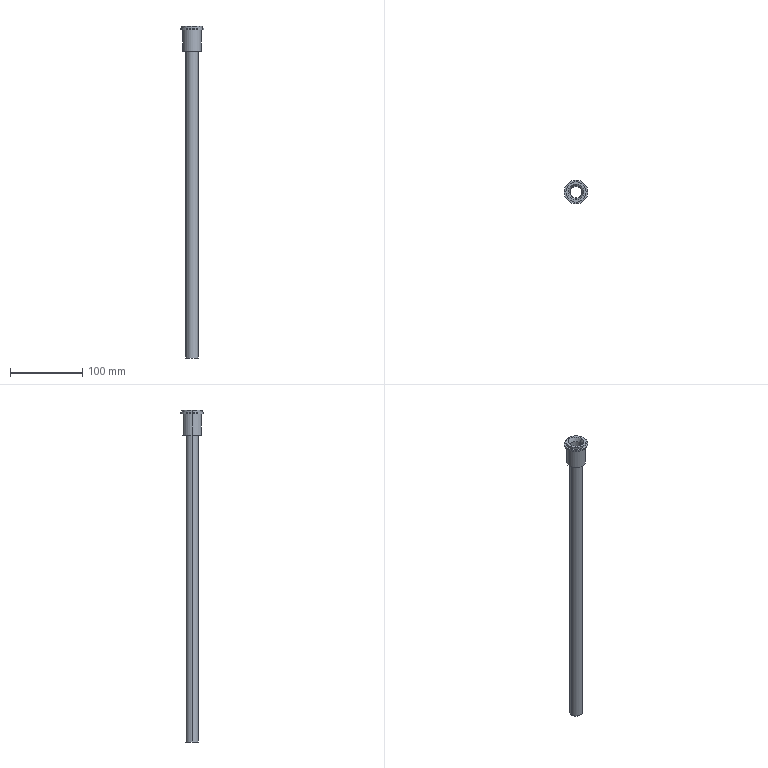Part | STEP file | Discharge pipe joint | 2 solids | 20 faces | box 33 x 33 x 460 mm | volume 22117 mm3 | cylinder 12 | plane 6 | cone 2 | commonest cylinder face diameters 17 x4 16 x2 26 x2 28 x2 33 x2
STEP:
#1=CARTESIAN_POINT('',(0.,0.,0.));
#2=DIRECTION('',(0.,0.,1.));
#3=DIRECTION('',(1.,0.,0.));
#4=AXIS2_PLACEMENT_3D('',#1,#2,#3);
#5=CARTESIAN_POINT('',(8.5,0.,-1.));
#6=VERTEX_POINT('',#5);
#7=CARTESIAN_POINT('',(11.,0.,5.));
#8=VERTEX_POINT('',#7);
#9=CARTESIAN_POINT('',(8.5,0.,-1.));
#10=DIRECTION('',(0.3846,0.,0.9231));
#11=VECTOR('',#10,1.);
#12=LINE('',#9,#11);
#13=CARTESIAN_POINT('',(0.,0.,-1.));
#14=DIRECTION('',(0.,0.,1.));
#15=DIRECTION('',(1.,0.,0.));
#16=AXIS2_PLACEMENT_3D('',#13,#14,#15);
#17=CONICAL_SURFACE('',#16,8.5,0.3948);
#18=CARTESIAN_POINT('',(6.283,0.));
#19=DIRECTION('',(0.,1.));
#20=VECTOR('',#19,1.);
#21=LINE('',#18,#20);
#22=(GEOMETRIC_REPRESENTATION_CONTEXT(2)PARAMETRIC_REPRESENTATION_CONTEXT()REPRESENTATION_CONTEXT('',''));
#23=DEFINITIONAL_REPRESENTATION('',(#21),#22);
#24=PCURVE('',#17,#23);
#25=CARTESIAN_POINT('',(0.,0.,-1.));
#26=DIRECTION('',(0.,0.,1.));
#27=DIRECTION('',(1.,0.,0.));
#28=AXIS2_PLACEMENT_3D('',#25,#26,#27);
#29=CONICAL_SURFACE('',#28,8.5,0.3948);
#30=CARTESIAN_POINT('',(0.,0.));
#31=DIRECTION('',(0.,1.));
#32=VECTOR('',#31,1.);
#33=LINE('',#30,#32);
#34=(GEOMETRIC_REPRESENTATION_CONTEXT(2)PARAMETRIC_REPRESENTATION_CONTEXT()REPRESENTATION_CONTEXT('',''));
#35=DEFINITIONAL_REPRESENTATION('',(#33),#34);
#36=PCURVE('',#29,#35);
#37=SURFACE_CURVE('',#12,(#24,#36),.PCURVE_S1.);
#38=EDGE_CURVE('',#6,#8,#37,.T.);
#39=ORIENTED_EDGE('',*,*,#38,.T.);
#40=CARTESIAN_POINT('',(-11.,0.,5.));
#41=VERTEX_POINT('',#40);
#42=CARTESIAN_POINT('',(0.,0.,5.));
#43=DIRECTION('',(0.,0.,1.));
#44=DIRECTION('',(1.,0.,0.));
#45=AXIS2_PLACEMENT_3D('',#42,#43,#44);
#46=CIRCLE('',#45,11.);
#47=CARTESIAN_POINT('',(0.,6.));
#48=DIRECTION('',(1.,0.));
#49=VECTOR('',#48,1.);
#50=LINE('',#47,#49);
#51=(GEOMETRIC_REPRESENTATION_CONTEXT(2)PARAMETRIC_REPRESENTATION_CONTEXT()REPRESENTATION_CONTEXT('',''));
#52=DEFINITIONAL_REPRESENTATION('',(#50),#51);
#53=PCURVE('',#17,#52);
#54=CARTESIAN_POINT('',(0.,0.,5.));
#55=DIRECTION('',(0.,0.,1.));
#56=DIRECTION('',(1.,0.,0.));
#57=AXIS2_PLACEMENT_3D('',#54,#55,#56);
#58=PLANE('',#57);
#59=CARTESIAN_POINT('',(0.,0.));
#60=DIRECTION('',(1.,0.));
#61=AXIS2_PLACEMENT_2D('',#59,#60);
#62=CIRCLE('',#61,11.);
#63=(GEOMETRIC_REPRESENTATION_CONTEXT(2)PARAMETRIC_REPRESENTATION_CONTEXT()REPRESENTATION_CONTEXT('',''));
#64=DEFINITIONAL_REPRESENTATION('',(#62),#63);
#65=PCURVE('',#58,#64);
#66=SURFACE_CURVE('',#46,(#53,#65),.PCURVE_S1.);
#67=EDGE_CURVE('',#41,#8,#66,.T.);
#68=ORIENTED_EDGE('',*,*,#67,.F.);
#69=CARTESIAN_POINT('',(-8.5,0.,-1.));
#70=VERTEX_POINT('',#69);
#71=CARTESIAN_POINT('',(-8.5,0.,-1.));
#72=DIRECTION('',(-0.3846,0.,0.9231));
#73=VECTOR('',#72,1.);
#74=LINE('',#71,#73);
#75=CARTESIAN_POINT('',(3.142,0.));
#76=DIRECTION('',(0.,1.));
#77=VECTOR('',#76,1.);
#78=LINE('',#75,#77);
#79=(GEOMETRIC_REPRESENTATION_CONTEXT(2)PARAMETRIC_REPRESENTATION_CONTEXT()REPRESENTATION_CONTEXT('',''));
#80=DEFINITIONAL_REPRESENTATION('',(#78),#79);
#81=PCURVE('',#17,#80);
#82=CARTESIAN_POINT('',(3.142,0.));
#83=DIRECTION('',(0.,1.));
#84=VECTOR('',#83,1.);
#85=LINE('',#82,#84);
#86=(GEOMETRIC_REPRESENTATION_CONTEXT(2)PARAMETRIC_REPRESENTATION_CONTEXT()REPRESENTATION_CONTEXT('',''));
#87=DEFINITIONAL_REPRESENTATION('',(#85),#86);
#88=PCURVE('',#29,#87);
#89=SURFACE_CURVE('',#74,(#81,#88),.PCURVE_S1.);
#90=EDGE_CURVE('',#70,#41,#89,.T.);
#91=ORIENTED_EDGE('',*,*,#90,.F.);
#92=CARTESIAN_POINT('',(0.,0.,-1.));
#93=DIRECTION('',(0.,0.,1.));
#94=DIRECTION('',(1.,0.,0.));
#95=AXIS2_PLACEMENT_3D('',#92,#93,#94);
#96=CIRCLE('',#95,8.5);
#97=CARTESIAN_POINT('',(0.,0.));
#98=DIRECTION('',(1.,0.));
#99=VECTOR('',#98,1.);
#100=LINE('',#97,#99);
#101=(GEOMETRIC_REPRESENTATION_CONTEXT(2)PARAMETRIC_REPRESENTATION_CONTEXT()REPRESENTATION_CONTEXT('',''));
#102=DEFINITIONAL_REPRESENTATION('',(#100),#101);
#103=PCURVE('',#17,#102);
#104=CARTESIAN_POINT('',(0.,0.,5.));
#105=DIRECTION('',(0.,0.,-1.));
#106=DIRECTION('',(-1.,0.,0.));
#107=AXIS2_PLACEMENT_3D('',#104,#105,#106);
#108=CYLINDRICAL_SURFACE('',#107,8.5);
#109=CARTESIAN_POINT('',(9.425,6.));
#110=DIRECTION('',(-1.,0.));
#111=VECTOR('',#110,1.);
#112=LINE('',#109,#111);
#113=(GEOMETRIC_REPRESENTATION_CONTEXT(2)PARAMETRIC_REPRESENTATION_CONTEXT()REPRESENTATION_CONTEXT('',''));
#114=DEFINITIONAL_REPRESENTATION('',(#112),#113);
#115=PCURVE('',#108,#114);
#116=SURFACE_CURVE('',#96,(#103,#115),.PCURVE_S1.);
#117=EDGE_CURVE('',#70,#6,#116,.T.);
#118=ORIENTED_EDGE('',*,*,#117,.T.);
#119=EDGE_LOOP('',(#39,#68,#91,#118));
#120=FACE_BOUND('',#119,.F.);
#121=ADVANCED_FACE('',(#120),#17,.F.);
#122=CARTESIAN_POINT('',(-13.,0.,-30.));
#123=VERTEX_POINT('',#122);
#124=CARTESIAN_POINT('',(13.,0.,-30.));
#125=VERTEX_POINT('',#124);
#126=CARTESIAN_POINT('',(0.,0.,-30.));
#127=DIRECTION('',(0.,0.,-1.));
#128=DIRECTION('',(-1.,0.,0.));
#129=AXIS2_PLACEMENT_3D('',#126,#127,#128);
#130=CIRCLE('',#129,13.);
#131=CARTESIAN_POINT('',(0.,0.,-30.));
#132=DIRECTION('',(0.,0.,1.));
#133=DIRECTION('',(1.,0.,0.));
#134=AXIS2_PLACEMENT_3D('',#131,#132,#133);
#135=CYLINDRICAL_SURFACE('',#134,13.);
#136=CARTESIAN_POINT('',(3.142,0.));
#137=DIRECTION('',(-1.,0.));
#138=VECTOR('',#137,1.);
#139=LINE('',#136,#138);
#140=(GEOMETRIC_REPRESENTATION_CONTEXT(2)PARAMETRIC_REPRESENTATION_CONTEXT()REPRESENTATION_CONTEXT('',''));
#141=DEFINITIONAL_REPRESENTATION('',(#139),#140);
#142=PCURVE('',#135,#141);
#143=CARTESIAN_POINT('',(0.,0.,-30.));
#144=DIRECTION('',(0.,0.,-1.));
#145=DIRECTION('',(-1.,0.,0.));
#146=AXIS2_PLACEMENT_3D('',#143,#144,#145);
#147=PLANE('',#146);
#148=CARTESIAN_POINT('',(0.,0.));
#149=DIRECTION('',(1.,0.));
#150=AXIS2_PLACEMENT_2D('',#148,#149);
#151=CIRCLE('',#150,13.);
#152=(GEOMETRIC_REPRESENTATION_CONTEXT(2)PARAMETRIC_REPRESENTATION_CONTEXT()REPRESENTATION_CONTEXT('',''));
#153=DEFINITIONAL_REPRESENTATION('',(#151),#152);
#154=PCURVE('',#147,#153);
#155=SURFACE_CURVE('',#130,(#142,#154),.PCURVE_S1.);
#156=EDGE_CURVE('',#123,#125,#155,.T.);
#157=ORIENTED_EDGE('',*,*,#156,.F.);
#158=CARTESIAN_POINT('',(-13.,0.,0.));
#159=VERTEX_POINT('',#158);
#160=CARTESIAN_POINT('',(-13.,0.,-30.));
#161=DIRECTION('',(0.,0.,1.));
#162=VECTOR('',#161,1.);
#163=LINE('',#160,#162);
#164=CARTESIAN_POINT('',(3.142,0.));
#165=DIRECTION('',(0.,1.));
#166=VECTOR('',#165,1.);
#167=LINE('',#164,#166);
#168=(GEOMETRIC_REPRESENTATION_CONTEXT(2)PARAMETRIC_REPRESENTATION_CONTEXT()REPRESENTATION_CONTEXT('',''));
#169=DEFINITIONAL_REPRESENTATION('',(#167),#168);
#170=PCURVE('',#135,#169);
#171=CARTESIAN_POINT('',(0.,0.,-30.));
#172=DIRECTION('',(0.,0.,1.));
#173=DIRECTION('',(1.,0.,0.));
#174=AXIS2_PLACEMENT_3D('',#171,#172,#173);
#175=CYLINDRICAL_SURFACE('',#174,13.);
#176=CARTESIAN_POINT('',(3.142,0.));
#177=DIRECTION('',(0.,1.));
#178=VECTOR('',#177,1.);
#179=LINE('',#176,#178);
#180=(GEOMETRIC_REPRESENTATION_CONTEXT(2)PARAMETRIC_REPRESENTATION_CONTEXT()REPRESENTATION_CONTEXT('',''));
#181=DEFINITIONAL_REPRESENTATION('',(#179),#180);
#182=PCURVE('',#175,#181);
#183=SURFACE_CURVE('',#163,(#170,#182),.PCURVE_S1.);
#184=EDGE_CURVE('',#123,#159,#183,.T.);
#185=ORIENTED_EDGE('',*,*,#184,.T.);
#186=CARTESIAN_POINT('',(13.,0.,0.));
#187=VERTEX_POINT('',#186);
#188=CARTESIAN_POINT('',(0.,0.,0.));
#189=DIRECTION('',(0.,0.,-1.));
#190=DIRECTION('',(-1.,0.,0.));
#191=AXIS2_PLACEMENT_3D('',#188,#189,#190);
#192=CIRCLE('',#191,13.);
#193=CARTESIAN_POINT('',(3.142,30.));
#194=DIRECTION('',(-1.,0.));
#195=VECTOR('',#194,1.);
#196=LINE('',#193,#195);
#197=(GEOMETRIC_REPRESENTATION_CONTEXT(2)PARAMETRIC_REPRESENTATION_CONTEXT()REPRESENTATION_CONTEXT('',''));
#198=DEFINITIONAL_REPRESENTATION('',(#196),#197);
#199=PCURVE('',#135,#198);
#200=CARTESIAN_POINT('',(0.,0.,0.));
#201=DIRECTION('',(0.,0.,1.));
#202=DIRECTION('',(1.,0.,0.));
#203=AXIS2_PLACEMENT_3D('',#200,#201,#202);
#204=PLANE('',#203);
#205=CARTESIAN_POINT('',(-13.,0.));
#206=CARTESIAN_POINT('',(-13.,22.517));
#207=CARTESIAN_POINT('',(6.5,11.258));
#208=CARTESIAN_POINT('',(26.,0.));
#209=CARTESIAN_POINT('',(6.5,-11.258));
#210=CARTESIAN_POINT('',(-13.,-22.517));
#211=CARTESIAN_POINT('',(-13.,0.));
#212=(BOUNDED_CURVE()B_SPLINE_CURVE(2,(#205,#206,#207,#208,#209,#210,#211),.UNSPECIFIED.,.T.,.F.)B_SPLINE_CURVE_WITH_KNOTS((1,2,2,2,2,1),(-2.094,0.,2.094,4.189,6.283,8.378),.UNSPECIFIED.)CURVE()GEOMETRIC_REPRESENTATION_ITEM()RATIONAL_B_SPLINE_CURVE((1.,0.5,1.,0.5,1.,0.5,1.))REPRESENTATION_ITEM(''));
#213=(GEOMETRIC_REPRESENTATION_CONTEXT(2)PARAMETRIC_REPRESENTATION_CONTEXT()REPRESENTATION_CONTEXT('',''));
#214=DEFINITIONAL_REPRESENTATION('',(#212),#213);
#215=PCURVE('',#204,#214);
#216=SURFACE_CURVE('',#192,(#199,#215),.PCURVE_S1.);
#217=EDGE_CURVE('',#159,#187,#216,.T.);
#218=ORIENTED_EDGE('',*,*,#217,.T.);
#219=CARTESIAN_POINT('',(13.,0.,-30.));
#220=DIRECTION('',(0.,0.,1.));
#221=VECTOR('',#220,1.);
#222=LINE('',#219,#221);
#223=CARTESIAN_POINT('',(0.,0.));
#224=DIRECTION('',(0.,1.));
#225=VECTOR('',#224,1.);
#226=LINE('',#223,#225);
#227=(GEOMETRIC_REPRESENTATION_CONTEXT(2)PARAMETRIC_REPRESENTATION_CONTEXT()REPRESENTATION_CONTEXT('',''));
#228=DEFINITIONAL_REPRESENTATION('',(#226),#227);
#229=PCURVE('',#135,#228);
#230=CARTESIAN_POINT('',(6.283,0.));
#231=DIRECTION('',(0.,1.));
#232=VECTOR('',#231,1.);
#233=LINE('',#230,#232);
#234=(GEOMETRIC_REPRESENTATION_CONTEXT(2)PARAMETRIC_REPRESENTATION_CONTEXT()REPRESENTATION_CONTEXT('',''));
#235=DEFINITIONAL_REPRESENTATION('',(#233),#234);
#236=PCURVE('',#175,#235);
#237=SURFACE_CURVE('',#222,(#229,#236),.PCURVE_S1.);
#238=EDGE_CURVE('',#125,#187,#237,.T.);
#239=ORIENTED_EDGE('',*,*,#238,.F.);
#240=EDGE_LOOP('',(#157,#185,#218,#239));
#241=FACE_BOUND('',#240,.T.);
#242=ADVANCED_FACE('',(#241),#135,.T.);
#243=CARTESIAN_POINT('',(14.,0.,5.));
#244=VERTEX_POINT('',#243);
#245=CARTESIAN_POINT('',(-14.,0.,5.));
#246=VERTEX_POINT('',#245);
#247=CARTESIAN_POINT('',(0.,0.,5.));
#248=DIRECTION('',(0.,0.,1.));
#249=DIRECTION('',(1.,0.,0.));
#250=AXIS2_PLACEMENT_3D('',#247,#248,#249);
#251=CIRCLE('',#250,14.);
#252=CARTESIAN_POINT('',(0.,0.,5.));
#253=DIRECTION('',(0.,0.,-1.));
#254=DIRECTION('',(-1.,0.,0.));
#255=AXIS2_PLACEMENT_3D('',#252,#253,#254);
#256=CYLINDRICAL_SURFACE('',#255,14.);
#257=CARTESIAN_POINT('',(3.142,0.));
#258=DIRECTION('',(-1.,0.));
#259=VECTOR('',#258,1.);
#260=LINE('',#257,#259);
#261=(GEOMETRIC_REPRESENTATION_CONTEXT(2)PARAMETRIC_REPRESENTATION_CONTEXT()REPRESENTATION_CONTEXT('',''));
#262=DEFINITIONAL_REPRESENTATION('',(#260),#261);
#263=PCURVE('',#256,#262);
#264=CARTESIAN_POINT('',(0.,0.));
#265=DIRECTION('',(1.,0.));
#266=AXIS2_PLACEMENT_2D('',#264,#265);
#267=CIRCLE('',#266,14.);
#268=(GEOMETRIC_REPRESENTATION_CONTEXT(2)PARAMETRIC_REPRESENTATION_CONTEXT()REPRESENTATION_CONTEXT('',''));
#269=DEFINITIONAL_REPRESENTATION('',(#267),#268);
#270=PCURVE('',#58,#269);
#271=SURFACE_CURVE('',#251,(#263,#270),.PCURVE_S1.);
#272=EDGE_CURVE('',#244,#246,#271,.T.);
#273=ORIENTED_EDGE('',*,*,#272,.F.);
#274=CARTESIAN_POINT('',(14.,0.,2.));
#275=VERTEX_POINT('',#274);
#276=CARTESIAN_POINT('',(14.,0.,5.));
#277=DIRECTION('',(0.,0.,-1.));
#278=VECTOR('',#277,1.);
#279=LINE('',#276,#278);
#280=CARTESIAN_POINT('',(3.142,0.));
#281=DIRECTION('',(0.,1.));
#282=VECTOR('',#281,1.);
#283=LINE('',#280,#282);
#284=(GEOMETRIC_REPRESENTATION_CONTEXT(2)PARAMETRIC_REPRESENTATION_CONTEXT()REPRESENTATION_CONTEXT('',''));
#285=DEFINITIONAL_REPRESENTATION('',(#283),#284);
#286=PCURVE('',#256,#285);
#287=CARTESIAN_POINT('',(0.,0.,5.));
#288=DIRECTION('',(0.,0.,-1.));
#289=DIRECTION('',(-1.,0.,0.));
#290=AXIS2_PLACEMENT_3D('',#287,#288,#289);
#291=CYLINDRICAL_SURFACE('',#290,14.);
#292=CARTESIAN_POINT('',(3.142,0.));
#293=DIRECTION('',(0.,1.));
#294=VECTOR('',#293,1.);
#295=LINE('',#292,#294);
#296=(GEOMETRIC_REPRESENTATION_CONTEXT(2)PARAMETRIC_REPRESENTATION_CONTEXT()REPRESENTATION_CONTEXT('',''));
#297=DEFINITIONAL_REPRESENTATION('',(#295),#296);
#298=PCURVE('',#291,#297);
#299=SURFACE_CURVE('',#279,(#286,#298),.PCURVE_S1.);
#300=EDGE_CURVE('',#244,#275,#299,.T.);
#301=ORIENTED_EDGE('',*,*,#300,.T.);
#302=CARTESIAN_POINT('',(-14.,0.,2.));
#303=VERTEX_POINT('',#302);
#304=CARTESIAN_POINT('',(0.,0.,2.));
#305=DIRECTION('',(0.,0.,1.));
#306=DIRECTION('',(1.,0.,0.));
#307=AXIS2_PLACEMENT_3D('',#304,#305,#306);
#308=CIRCLE('',#307,14.);
#309=CARTESIAN_POINT('',(3.142,3.));
#310=DIRECTION('',(-1.,0.));
#311=VECTOR('',#310,1.);
#312=LINE('',#309,#311);
#313=(GEOMETRIC_REPRESENTATION_CONTEXT(2)PARAMETRIC_REPRESENTATION_CONTEXT()REPRESENTATION_CONTEXT('',''));
#314=DEFINITIONAL_REPRESENTATION('',(#312),#313);
#315=PCURVE('',#256,#314);
#316=CARTESIAN_POINT('',(0.,0.,2.));
#317=DIRECTION('',(0.,0.,1.));
#318=DIRECTION('',(1.,0.,0.));
#319=AXIS2_PLACEMENT_3D('',#316,#317,#318);
#320=PLANE('',#319);
#321=CARTESIAN_POINT('',(0.,0.));
#322=DIRECTION('',(1.,0.));
#323=AXIS2_PLACEMENT_2D('',#321,#322);
#324=CIRCLE('',#323,14.);
#325=(GEOMETRIC_REPRESENTATION_CONTEXT(2)PARAMETRIC_REPRESENTATION_CONTEXT()REPRESENTATION_CONTEXT('',''));
#326=DEFINITIONAL_REPRESENTATION('',(#324),#325);
#327=PCURVE('',#320,#326);
#328=SURFACE_CURVE('',#308,(#315,#327),.PCURVE_S1.);
#329=EDGE_CURVE('',#275,#303,#328,.T.);
#330=ORIENTED_EDGE('',*,*,#329,.T.);
#331=CARTESIAN_POINT('',(-14.,0.,5.));
#332=DIRECTION('',(0.,0.,-1.));
#333=VECTOR('',#332,1.);
#334=LINE('',#331,#333);
#335=CARTESIAN_POINT('',(0.,0.));
#336=DIRECTION('',(0.,1.));
#337=VECTOR('',#336,1.);
#338=LINE('',#335,#337);
#339=(GEOMETRIC_REPRESENTATION_CONTEXT(2)PARAMETRIC_REPRESENTATION_CONTEXT()REPRESENTATION_CONTEXT('',''));
#340=DEFINITIONAL_REPRESENTATION('',(#338),#339);
#341=PCURVE('',#256,#340);
#342=CARTESIAN_POINT('',(6.283,0.));
#343=DIRECTION('',(0.,1.));
#344=VECTOR('',#343,1.);
#345=LINE('',#342,#344);
#346=(GEOMETRIC_REPRESENTATION_CONTEXT(2)PARAMETRIC_REPRESENTATION_CONTEXT()REPRESENTATION_CONTEXT('',''));
#347=DEFINITIONAL_REPRESENTATION('',(#345),#346);
#348=PCURVE('',#291,#347);
#349=SURFACE_CURVE('',#334,(#341,#348),.PCURVE_S1.);
#350=EDGE_CURVE('',#246,#303,#349,.T.);
#351=ORIENTED_EDGE('',*,*,#350,.F.);
#352=EDGE_LOOP('',(#273,#301,#330,#351));
#353=FACE_BOUND('',#352,.T.);
#354=ADVANCED_FACE('',(#353),#256,.T.);
#355=CARTESIAN_POINT('',(16.5,0.,2.));
#356=VERTEX_POINT('',#355);
#357=CARTESIAN_POINT('',(-16.5,0.,2.));
#358=VERTEX_POINT('',#357);
#359=CARTESIAN_POINT('',(0.,0.,2.));
#360=DIRECTION('',(0.,0.,1.));
#361=DIRECTION('',(1.,0.,0.));
#362=AXIS2_PLACEMENT_3D('',#359,#360,#361);
#363=CIRCLE('',#362,16.5);
#364=CARTESIAN_POINT('',(0.,0.,2.));
#365=DIRECTION('',(0.,0.,-1.));
#366=DIRECTION('',(-1.,0.,0.));
#367=AXIS2_PLACEMENT_3D('',#364,#365,#366);
#368=CYLINDRICAL_SURFACE('',#367,16.5);
#369=CARTESIAN_POINT('',(3.142,0.));
#370=DIRECTION('',(-1.,0.));
#371=VECTOR('',#370,1.);
#372=LINE('',#369,#371);
#373=(GEOMETRIC_REPRESENTATION_CONTEXT(2)PARAMETRIC_REPRESENTATION_CONTEXT()REPRESENTATION_CONTEXT('',''));
#374=DEFINITIONAL_REPRESENTATION('',(#372),#373);
#375=PCURVE('',#368,#374);
#376=CARTESIAN_POINT('',(0.,0.));
#377=DIRECTION('',(1.,0.));
#378=AXIS2_PLACEMENT_2D('',#376,#377);
#379=CIRCLE('',#378,16.5);
#380=(GEOMETRIC_REPRESENTATION_CONTEXT(2)PARAMETRIC_REPRESENTATION_CONTEXT()REPRESENTATION_CONTEXT('',''));
#381=DEFINITIONAL_REPRESENTATION('',(#379),#380);
#382=PCURVE('',#320,#381);
#383=SURFACE_CURVE('',#363,(#375,#382),.PCURVE_S1.);
#384=EDGE_CURVE('',#356,#358,#383,.T.);
#385=ORIENTED_EDGE('',*,*,#384,.F.);
#386=CARTESIAN_POINT('',(16.5,0.,0.));
#387=VERTEX_POINT('',#386);
#388=CARTESIAN_POINT('',(16.5,0.,2.));
#389=DIRECTION('',(0.,0.,-1.));
#390=VECTOR('',#389,1.);
#391=LINE('',#388,#390);
#392=CARTESIAN_POINT('',(3.142,0.));
#393=DIRECTION('',(0.,1.));
#394=VECTOR('',#393,1.);
#395=LINE('',#392,#394);
#396=(GEOMETRIC_REPRESENTATION_CONTEXT(2)PARAMETRIC_REPRESENTATION_CONTEXT()REPRESENTATION_CONTEXT('',''));
#397=DEFINITIONAL_REPRESENTATION('',(#395),#396);
#398=PCURVE('',#368,#397);
#399=CARTESIAN_POINT('',(0.,0.,2.));
#400=DIRECTION('',(0.,0.,-1.));
#401=DIRECTION('',(-1.,0.,0.));
#402=AXIS2_PLACEMENT_3D('',#399,#400,#401);
#403=CYLINDRICAL_SURFACE('',#402,16.5);
#404=CARTESIAN_POINT('',(3.142,0.));
#405=DIRECTION('',(0.,1.));
#406=VECTOR('',#405,1.);
#407=LINE('',#404,#406);
#408=(GEOMETRIC_REPRESENTATION_CONTEXT(2)PARAMETRIC_REPRESENTATION_CONTEXT()REPRESENTATION_CONTEXT('',''));
#409=DEFINITIONAL_REPRESENTATION('',(#407),#408);
#410=PCURVE('',#403,#409);
#411=SURFACE_CURVE('',#391,(#398,#410),.PCURVE_S1.);
#412=EDGE_CURVE('',#356,#387,#411,.T.);
#413=ORIENTED_EDGE('',*,*,#412,.T.);
#414=CARTESIAN_POINT('',(-16.5,0.,0.));
#415=VERTEX_POINT('',#414);
#416=CARTESIAN_POINT('',(0.,0.,0.));
#417=DIRECTION('',(0.,0.,1.));
#418=DIRECTION('',(1.,0.,0.));
#419=AXIS2_PLACEMENT_3D('',#416,#417,#418);
#420=CIRCLE('',#419,16.5);
#421=CARTESIAN_POINT('',(3.142,2.));
#422=DIRECTION('',(-1.,0.));
#423=VECTOR('',#422,1.);
#424=LINE('',#421,#423);
#425=(GEOMETRIC_REPRESENTATION_CONTEXT(2)PARAMETRIC_REPRESENTATION_CONTEXT()REPRESENTATION_CONTEXT('',''));
#426=DEFINITIONAL_REPRESENTATION('',(#424),#425);
#427=PCURVE('',#368,#426);
#428=CARTESIAN_POINT('',(0.,0.));
#429=DIRECTION('',(1.,0.));
#430=AXIS2_PLACEMENT_2D('',#428,#429);
#431=CIRCLE('',#430,16.5);
#432=(GEOMETRIC_REPRESENTATION_CONTEXT(2)PARAMETRIC_REPRESENTATION_CONTEXT()REPRESENTATION_CONTEXT('',''));
#433=DEFINITIONAL_REPRESENTATION('',(#431),#432);
#434=PCURVE('',#204,#433);
#435=SURFACE_CURVE('',#420,(#427,#434),.PCURVE_S1.);
#436=EDGE_CURVE('',#387,#415,#435,.T.);
#437=ORIENTED_EDGE('',*,*,#436,.T.);
#438=CARTESIAN_POINT('',(-16.5,0.,2.));
#439=DIRECTION('',(0.,0.,-1.));
#440=VECTOR('',#439,1.);
#441=LINE('',#438,#440);
#442=CARTESIAN_POINT('',(0.,0.));
#443=DIRECTION('',(0.,1.));
#444=VECTOR('',#443,1.);
#445=LINE('',#442,#444);
#446=(GEOMETRIC_REPRESENTATION_CONTEXT(2)PARAMETRIC_REPRESENTATION_CONTEXT()REPRESENTATION_CONTEXT('',''));
#447=DEFINITIONAL_REPRESENTATION('',(#445),#446);
#448=PCURVE('',#368,#447);
#449=CARTESIAN_POINT('',(6.283,0.));
#450=DIRECTION('',(0.,1.));
#451=VECTOR('',#450,1.);
#452=LINE('',#449,#451);
#453=(GEOMETRIC_REPRESENTATION_CONTEXT(2)PARAMETRIC_REPRESENTATION_CONTEXT()REPRESENTATION_CONTEXT('',''));
#454=DEFINITIONAL_REPRESENTATION('',(#452),#453);
#455=PCURVE('',#403,#454);
#456=SURFACE_CURVE('',#441,(#448,#455),.PCURVE_S1.);
#457=EDGE_CURVE('',#358,#415,#456,.T.);
#458=ORIENTED_EDGE('',*,*,#457,.F.);
#459=EDGE_LOOP('',(#385,#413,#437,#458));
#460=FACE_BOUND('',#459,.T.);
#461=ADVANCED_FACE('',(#460),#368,.T.);
#462=CARTESIAN_POINT('',(-8.5,0.,-30.));
#463=VERTEX_POINT('',#462);
#464=CARTESIAN_POINT('',(-8.5,0.,5.));
#465=DIRECTION('',(0.,0.,-1.));
#466=VECTOR('',#465,1.);
#467=LINE('',#464,#466);
#468=CARTESIAN_POINT('',(6.283,0.));
#469=DIRECTION('',(0.,1.));
#470=VECTOR('',#469,1.);
#471=LINE('',#468,#470);
#472=(GEOMETRIC_REPRESENTATION_CONTEXT(2)PARAMETRIC_REPRESENTATION_CONTEXT()REPRESENTATION_CONTEXT('',''));
#473=DEFINITIONAL_REPRESENTATION('',(#471),#472);
#474=PCURVE('',#108,#473);
#475=CARTESIAN_POINT('',(0.,0.,5.));
#476=DIRECTION('',(0.,0.,-1.));
#477=DIRECTION('',(-1.,0.,0.));
#478=AXIS2_PLACEMENT_3D('',#475,#476,#477);
#479=CYLINDRICAL_SURFACE('',#478,8.5);
#480=CARTESIAN_POINT('',(0.,0.));
#481=DIRECTION('',(0.,1.));
#482=VECTOR('',#481,1.);
#483=LINE('',#480,#482);
#484=(GEOMETRIC_REPRESENTATION_CONTEXT(2)PARAMETRIC_REPRESENTATION_CONTEXT()REPRESENTATION_CONTEXT('',''));
#485=DEFINITIONAL_REPRESENTATION('',(#483),#484);
#486=PCURVE('',#479,#485);
#487=SURFACE_CURVE('',#467,(#474,#486),.PCURVE_S1.);
#488=EDGE_CURVE('',#70,#463,#487,.T.);
#489=ORIENTED_EDGE('',*,*,#488,.T.);
#490=CARTESIAN_POINT('',(8.5,0.,-30.));
#491=VERTEX_POINT('',#490);
#492=CARTESIAN_POINT('',(0.,0.,-30.));
#493=DIRECTION('',(0.,0.,-1.));
#494=DIRECTION('',(-1.,0.,0.));
#495=AXIS2_PLACEMENT_3D('',#492,#493,#494);
#496=CIRCLE('',#495,8.5);
#497=CARTESIAN_POINT('',(0.,35.));
#498=DIRECTION('',(1.,0.));
#499=VECTOR('',#498,1.);
#500=LINE('',#497,#499);
#501=(GEOMETRIC_REPRESENTATION_CONTEXT(2)PARAMETRIC_REPRESENTATION_CONTEXT()REPRESENTATION_CONTEXT('',''));
#502=DEFINITIONAL_REPRESENTATION('',(#500),#501);
#503=PCURVE('',#108,#502);
#504=CARTESIAN_POINT('',(0.,0.));
#505=DIRECTION('',(1.,0.));
#506=AXIS2_PLACEMENT_2D('',#504,#505);
#507=CIRCLE('',#506,8.5);
#508=(GEOMETRIC_REPRESENTATION_CONTEXT(2)PARAMETRIC_REPRESENTATION_CONTEXT()REPRESENTATION_CONTEXT('',''));
#509=DEFINITIONAL_REPRESENTATION('',(#507),#508);
#510=PCURVE('',#147,#509);
#511=SURFACE_CURVE('',#496,(#503,#510),.PCURVE_S1.);
#512=EDGE_CURVE('',#491,#463,#511,.T.);
#513=ORIENTED_EDGE('',*,*,#512,.F.);
#514=CARTESIAN_POINT('',(8.5,0.,5.));
#515=DIRECTION('',(0.,0.,-1.));
#516=VECTOR('',#515,1.);
#517=LINE('',#514,#516);
#518=CARTESIAN_POINT('',(3.142,0.));
#519=DIRECTION('',(0.,1.));
#520=VECTOR('',#519,1.);
#521=LINE('',#518,#520);
#522=(GEOMETRIC_REPRESENTATION_CONTEXT(2)PARAMETRIC_REPRESENTATION_CONTEXT()REPRESENTATION_CONTEXT('',''));
#523=DEFINITIONAL_REPRESENTATION('',(#521),#522);
#524=PCURVE('',#108,#523);
#525=CARTESIAN_POINT('',(3.142,0.));
#526=DIRECTION('',(0.,1.));
#527=VECTOR('',#526,1.);
#528=LINE('',#525,#527);
#529=(GEOMETRIC_REPRESENTATION_CONTEXT(2)PARAMETRIC_REPRESENTATION_CONTEXT()REPRESENTATION_CONTEXT('',''));
#530=DEFINITIONAL_REPRESENTATION('',(#528),#529);
#531=PCURVE('',#479,#530);
#532=SURFACE_CURVE('',#517,(#524,#531),.PCURVE_S1.);
#533=EDGE_CURVE('',#6,#491,#532,.T.);
#534=ORIENTED_EDGE('',*,*,#533,.F.);
#535=ORIENTED_EDGE('',*,*,#117,.F.);
#536=EDGE_LOOP('',(#489,#513,#534,#535));
#537=FACE_BOUND('',#536,.F.);
#538=ADVANCED_FACE('',(#537),#108,.F.);
#539=CARTESIAN_POINT('',(0.,0.,-30.));
#540=DIRECTION('',(0.,0.,-1.));
#541=DIRECTION('',(-1.,0.,0.));
#542=AXIS2_PLACEMENT_3D('',#539,#540,#541);
#543=CIRCLE('',#542,8.5);
#544=CARTESIAN_POINT('',(0.,35.));
#545=DIRECTION('',(1.,0.));
#546=VECTOR('',#545,1.);
#547=LINE('',#544,#546);
#548=(GEOMETRIC_REPRESENTATION_CONTEXT(2)PARAMETRIC_REPRESENTATION_CONTEXT()REPRESENTATION_CONTEXT('',''));
#549=DEFINITIONAL_REPRESENTATION('',(#547),#548);
#550=PCURVE('',#479,#549);
#551=CARTESIAN_POINT('',(0.,0.));
#552=DIRECTION('',(1.,0.));
#553=AXIS2_PLACEMENT_2D('',#551,#552);
#554=CIRCLE('',#553,8.5);
#555=(GEOMETRIC_REPRESENTATION_CONTEXT(2)PARAMETRIC_REPRESENTATION_CONTEXT()REPRESENTATION_CONTEXT('',''));
#556=DEFINITIONAL_REPRESENTATION('',(#554),#555);
#557=PCURVE('',#147,#556);
#558=SURFACE_CURVE('',#543,(#550,#557),.PCURVE_S1.);
#559=EDGE_CURVE('',#463,#491,#558,.T.);
#560=ORIENTED_EDGE('',*,*,#559,.F.);
#561=ORIENTED_EDGE('',*,*,#488,.F.);
#562=CARTESIAN_POINT('',(0.,0.,-1.));
#563=DIRECTION('',(0.,0.,1.));
#564=DIRECTION('',(1.,0.,0.));
#565=AXIS2_PLACEMENT_3D('',#562,#563,#564);
#566=CIRCLE('',#565,8.5);
#567=CARTESIAN_POINT('',(3.142,6.));
#568=DIRECTION('',(-1.,0.));
#569=VECTOR('',#568,1.);
#570=LINE('',#567,#569);
#571=(GEOMETRIC_REPRESENTATION_CONTEXT(2)PARAMETRIC_REPRESENTATION_CONTEXT()REPRESENTATION_CONTEXT('',''));
#572=DEFINITIONAL_REPRESENTATION('',(#570),#571);
#573=PCURVE('',#479,#572);
#574=CARTESIAN_POINT('',(0.,0.));
#575=DIRECTION('',(1.,0.));
#576=VECTOR('',#575,1.);
#577=LINE('',#574,#576);
#578=(GEOMETRIC_REPRESENTATION_CONTEXT(2)PARAMETRIC_REPRESENTATION_CONTEXT()REPRESENTATION_CONTEXT('',''));
#579=DEFINITIONAL_REPRESENTATION('',(#577),#578);
#580=PCURVE('',#29,#579);
#581=SURFACE_CURVE('',#566,(#573,#580),.PCURVE_S1.);
#582=EDGE_CURVE('',#6,#70,#581,.T.);
#583=ORIENTED_EDGE('',*,*,#582,.F.);
#584=ORIENTED_EDGE('',*,*,#533,.T.);
#585=EDGE_LOOP('',(#560,#561,#583,#584));
#586=FACE_BOUND('',#585,.F.);
#587=ADVANCED_FACE('',(#586),#479,.F.);
#588=ORIENTED_EDGE('',*,*,#412,.F.);
#589=CARTESIAN_POINT('',(0.,0.,2.));
#590=DIRECTION('',(0.,0.,1.));
#591=DIRECTION('',(1.,0.,0.));
#592=AXIS2_PLACEMENT_3D('',#589,#590,#591);
#593=CIRCLE('',#592,16.5);
#594=CARTESIAN_POINT('',(9.425,0.));
#595=DIRECTION('',(-1.,0.));
#596=VECTOR('',#595,1.);
#597=LINE('',#594,#596);
#598=(GEOMETRIC_REPRESENTATION_CONTEXT(2)PARAMETRIC_REPRESENTATION_CONTEXT()REPRESENTATION_CONTEXT('',''));
#599=DEFINITIONAL_REPRESENTATION('',(#597),#598);
#600=PCURVE('',#403,#599);
#601=CARTESIAN_POINT('',(0.,0.));
#602=DIRECTION('',(1.,0.));
#603=AXIS2_PLACEMENT_2D('',#601,#602);
#604=CIRCLE('',#603,16.5);
#605=(GEOMETRIC_REPRESENTATION_CONTEXT(2)PARAMETRIC_REPRESENTATION_CONTEXT()REPRESENTATION_CONTEXT('',''));
#606=DEFINITIONAL_REPRESENTATION('',(#604),#605);
#607=PCURVE('',#320,#606);
#608=SURFACE_CURVE('',#593,(#600,#607),.PCURVE_S1.);
#609=EDGE_CURVE('',#358,#356,#608,.T.);
#610=ORIENTED_EDGE('',*,*,#609,.F.);
#611=ORIENTED_EDGE('',*,*,#457,.T.);
#612=CARTESIAN_POINT('',(0.,0.,0.));
#613=DIRECTION('',(0.,0.,1.));
#614=DIRECTION('',(1.,0.,0.));
#615=AXIS2_PLACEMENT_3D('',#612,#613,#614);
#616=CIRCLE('',#615,16.5);
#617=CARTESIAN_POINT('',(9.425,2.));
#618=DIRECTION('',(-1.,0.));
#619=VECTOR('',#618,1.);
#620=LINE('',#617,#619);
#621=(GEOMETRIC_REPRESENTATION_CONTEXT(2)PARAMETRIC_REPRESENTATION_CONTEXT()REPRESENTATION_CONTEXT('',''));
#622=DEFINITIONAL_REPRESENTATION('',(#620),#621);
#623=PCURVE('',#403,#622);
#624=CARTESIAN_POINT('',(0.,0.));
#625=DIRECTION('',(1.,0.));
#626=AXIS2_PLACEMENT_2D('',#624,#625);
#627=CIRCLE('',#626,16.5);
#628=(GEOMETRIC_REPRESENTATION_CONTEXT(2)PARAMETRIC_REPRESENTATION_CONTEXT()REPRESENTATION_CONTEXT('',''));
#629=DEFINITIONAL_REPRESENTATION('',(#627),#628);
#630=PCURVE('',#204,#629);
#631=SURFACE_CURVE('',#616,(#623,#630),.PCURVE_S1.);
#632=EDGE_CURVE('',#415,#387,#631,.T.);
#633=ORIENTED_EDGE('',*,*,#632,.T.);
#634=EDGE_LOOP('',(#588,#610,#611,#633));
#635=FACE_BOUND('',#634,.T.);
#636=ADVANCED_FACE('',(#635),#403,.T.);
#637=CARTESIAN_POINT('',(0.,0.,2.));
#638=DIRECTION('',(0.,0.,1.));
#639=DIRECTION('',(1.,0.,0.));
#640=AXIS2_PLACEMENT_3D('',#637,#638,#639);
#641=CIRCLE('',#640,14.);
#642=CARTESIAN_POINT('',(0.,0.));
#643=DIRECTION('',(1.,0.));
#644=AXIS2_PLACEMENT_2D('',#642,#643);
#645=CIRCLE('',#644,14.);
#646=(GEOMETRIC_REPRESENTATION_CONTEXT(2)PARAMETRIC_REPRESENTATION_CONTEXT()REPRESENTATION_CONTEXT('',''));
#647=DEFINITIONAL_REPRESENTATION('',(#645),#646);
#648=PCURVE('',#320,#647);
#649=CARTESIAN_POINT('',(9.425,3.));
#650=DIRECTION('',(-1.,0.));
#651=VECTOR('',#650,1.);
#652=LINE('',#649,#651);
#653=(GEOMETRIC_REPRESENTATION_CONTEXT(2)PARAMETRIC_REPRESENTATION_CONTEXT()REPRESENTATION_CONTEXT('',''));
#654=DEFINITIONAL_REPRESENTATION('',(#652),#653);
#655=PCURVE('',#291,#654);
#656=SURFACE_CURVE('',#641,(#648,#655),.PCURVE_S1.);
#657=EDGE_CURVE('',#303,#275,#656,.T.);
#658=ORIENTED_EDGE('',*,*,#657,.F.);
#659=ORIENTED_EDGE('',*,*,#329,.F.);
#660=EDGE_LOOP('',(#658,#659));
#661=FACE_BOUND('',#660,.T.);
#662=ORIENTED_EDGE('',*,*,#609,.T.);
#663=ORIENTED_EDGE('',*,*,#384,.T.);
#664=EDGE_LOOP('',(#662,#663));
#665=FACE_BOUND('',#664,.T.);
#666=ADVANCED_FACE('',(#661,#665),#320,.T.);
#667=CARTESIAN_POINT('',(0.,0.,0.));
#668=DIRECTION('',(0.,0.,-1.));
#669=DIRECTION('',(-1.,0.,0.));
#670=AXIS2_PLACEMENT_3D('',#667,#668,#669);
#671=CIRCLE('',#670,13.);
#672=CARTESIAN_POINT('',(-13.,0.));
#673=CARTESIAN_POINT('',(-13.,22.517));
#674=CARTESIAN_POINT('',(6.5,11.258));
#675=CARTESIAN_POINT('',(26.,0.));
#676=CARTESIAN_POINT('',(6.5,-11.258));
#677=CARTESIAN_POINT('',(-13.,-22.517));
#678=CARTESIAN_POINT('',(-13.,0.));
#679=(BOUNDED_CURVE()B_SPLINE_CURVE(2,(#672,#673,#674,#675,#676,#677,#678),.UNSPECIFIED.,.T.,.F.)B_SPLINE_CURVE_WITH_KNOTS((1,2,2,2,2,1),(-2.094,0.,2.094,4.189,6.283,8.378),.UNSPECIFIED.)CURVE()GEOMETRIC_REPRESENTATION_ITEM()RATIONAL_B_SPLINE_CURVE((1.,0.5,1.,0.5,1.,0.5,1.))REPRESENTATION_ITEM(''));
#680=(GEOMETRIC_REPRESENTATION_CONTEXT(2)PARAMETRIC_REPRESENTATION_CONTEXT()REPRESENTATION_CONTEXT('',''));
#681=DEFINITIONAL_REPRESENTATION('',(#679),#680);
#682=PCURVE('',#204,#681);
#683=CARTESIAN_POINT('',(9.425,30.));
#684=DIRECTION('',(-1.,0.));
#685=VECTOR('',#684,1.);
#686=LINE('',#683,#685);
#687=(GEOMETRIC_REPRESENTATION_CONTEXT(2)PARAMETRIC_REPRESENTATION_CONTEXT()REPRESENTATION_CONTEXT('',''));
#688=DEFINITIONAL_REPRESENTATION('',(#686),#687);
#689=PCURVE('',#175,#688);
#690=SURFACE_CURVE('',#671,(#682,#689),.PCURVE_S1.);
#691=EDGE_CURVE('',#187,#159,#690,.T.);
#692=ORIENTED_EDGE('',*,*,#691,.F.);
#693=ORIENTED_EDGE('',*,*,#217,.F.);
#694=EDGE_LOOP('',(#692,#693));
#695=FACE_BOUND('',#694,.T.);
#696=ORIENTED_EDGE('',*,*,#632,.F.);
#697=ORIENTED_EDGE('',*,*,#436,.F.);
#698=EDGE_LOOP('',(#696,#697));
#699=FACE_BOUND('',#698,.T.);
#700=ADVANCED_FACE('',(#695,#699),#204,.F.);
#701=ORIENTED_EDGE('',*,*,#300,.F.);
#702=CARTESIAN_POINT('',(0.,0.,5.));
#703=DIRECTION('',(0.,0.,1.));
#704=DIRECTION('',(1.,0.,0.));
#705=AXIS2_PLACEMENT_3D('',#702,#703,#704);
#706=CIRCLE('',#705,14.);
#707=CARTESIAN_POINT('',(9.425,0.));
#708=DIRECTION('',(-1.,0.));
#709=VECTOR('',#708,1.);
#710=LINE('',#707,#709);
#711=(GEOMETRIC_REPRESENTATION_CONTEXT(2)PARAMETRIC_REPRESENTATION_CONTEXT()REPRESENTATION_CONTEXT('',''));
#712=DEFINITIONAL_REPRESENTATION('',(#710),#711);
#713=PCURVE('',#291,#712);
#714=CARTESIAN_POINT('',(0.,0.));
#715=DIRECTION('',(1.,0.));
#716=AXIS2_PLACEMENT_2D('',#714,#715);
#717=CIRCLE('',#716,14.);
#718=(GEOMETRIC_REPRESENTATION_CONTEXT(2)PARAMETRIC_REPRESENTATION_CONTEXT()REPRESENTATION_CONTEXT('',''));
#719=DEFINITIONAL_REPRESENTATION('',(#717),#718);
#720=PCURVE('',#58,#719);
#721=SURFACE_CURVE('',#706,(#713,#720),.PCURVE_S1.);
#722=EDGE_CURVE('',#246,#244,#721,.T.);
#723=ORIENTED_EDGE('',*,*,#722,.F.);
#724=ORIENTED_EDGE('',*,*,#350,.T.);
#725=ORIENTED_EDGE('',*,*,#657,.T.);
#726=EDGE_LOOP('',(#701,#723,#724,#725));
#727=FACE_BOUND('',#726,.T.);
#728=ADVANCED_FACE('',(#727),#291,.T.);
#729=CARTESIAN_POINT('',(0.,0.,5.));
#730=DIRECTION('',(0.,0.,1.));
#731=DIRECTION('',(1.,0.,0.));
#732=AXIS2_PLACEMENT_3D('',#729,#730,#731);
#733=CIRCLE('',#732,11.);
#734=CARTESIAN_POINT('',(0.,0.));
#735=DIRECTION('',(1.,0.));
#736=AXIS2_PLACEMENT_2D('',#734,#735);
#737=CIRCLE('',#736,11.);
#738=(GEOMETRIC_REPRESENTATION_CONTEXT(2)PARAMETRIC_REPRESENTATION_CONTEXT()REPRESENTATION_CONTEXT('',''));
#739=DEFINITIONAL_REPRESENTATION('',(#737),#738);
#740=PCURVE('',#58,#739);
#741=CARTESIAN_POINT('',(0.,6.));
#742=DIRECTION('',(1.,0.));
#743=VECTOR('',#742,1.);
#744=LINE('',#741,#743);
#745=(GEOMETRIC_REPRESENTATION_CONTEXT(2)PARAMETRIC_REPRESENTATION_CONTEXT()REPRESENTATION_CONTEXT('',''));
#746=DEFINITIONAL_REPRESENTATION('',(#744),#745);
#747=PCURVE('',#29,#746);
#748=SURFACE_CURVE('',#733,(#740,#747),.PCURVE_S1.);
#749=EDGE_CURVE('',#8,#41,#748,.T.);
#750=ORIENTED_EDGE('',*,*,#749,.F.);
#751=ORIENTED_EDGE('',*,*,#67,.F.);
#752=EDGE_LOOP('',(#750,#751));
#753=FACE_BOUND('',#752,.T.);
#754=ORIENTED_EDGE('',*,*,#722,.T.);
#755=ORIENTED_EDGE('',*,*,#272,.T.);
#756=EDGE_LOOP('',(#754,#755));
#757=FACE_BOUND('',#756,.T.);
#758=ADVANCED_FACE('',(#753,#757),#58,.T.);
#759=ORIENTED_EDGE('',*,*,#184,.F.);
#760=CARTESIAN_POINT('',(0.,0.,-30.));
#761=DIRECTION('',(0.,0.,-1.));
#762=DIRECTION('',(-1.,0.,0.));
#763=AXIS2_PLACEMENT_3D('',#760,#761,#762);
#764=CIRCLE('',#763,13.);
#765=CARTESIAN_POINT('',(9.425,0.));
#766=DIRECTION('',(-1.,0.));
#767=VECTOR('',#766,1.);
#768=LINE('',#765,#767);
#769=(GEOMETRIC_REPRESENTATION_CONTEXT(2)PARAMETRIC_REPRESENTATION_CONTEXT()REPRESENTATION_CONTEXT('',''));
#770=DEFINITIONAL_REPRESENTATION('',(#768),#769);
#771=PCURVE('',#175,#770);
#772=CARTESIAN_POINT('',(0.,0.));
#773=DIRECTION('',(1.,0.));
#774=AXIS2_PLACEMENT_2D('',#772,#773);
#775=CIRCLE('',#774,13.);
#776=(GEOMETRIC_REPRESENTATION_CONTEXT(2)PARAMETRIC_REPRESENTATION_CONTEXT()REPRESENTATION_CONTEXT('',''));
#777=DEFINITIONAL_REPRESENTATION('',(#775),#776);
#778=PCURVE('',#147,#777);
#779=SURFACE_CURVE('',#764,(#771,#778),.PCURVE_S1.);
#780=EDGE_CURVE('',#125,#123,#779,.T.);
#781=ORIENTED_EDGE('',*,*,#780,.F.);
#782=ORIENTED_EDGE('',*,*,#238,.T.);
#783=ORIENTED_EDGE('',*,*,#691,.T.);
#784=EDGE_LOOP('',(#759,#781,#782,#783));
#785=FACE_BOUND('',#784,.T.);
#786=ADVANCED_FACE('',(#785),#175,.T.);
#787=ORIENTED_EDGE('',*,*,#559,.F.);
#788=ORIENTED_EDGE('',*,*,#512,.F.);
#789=EDGE_LOOP('',(#787,#788));
#790=FACE_BOUND('',#789,.T.);
#791=ORIENTED_EDGE('',*,*,#780,.T.);
#792=ORIENTED_EDGE('',*,*,#156,.T.);
#793=EDGE_LOOP('',(#791,#792));
#794=FACE_BOUND('',#793,.T.);
#795=ADVANCED_FACE('',(#790,#794),#147,.T.);
#796=ORIENTED_EDGE('',*,*,#749,.F.);
#797=ORIENTED_EDGE('',*,*,#38,.F.);
#798=ORIENTED_EDGE('',*,*,#582,.T.);
#799=ORIENTED_EDGE('',*,*,#90,.T.);
#800=EDGE_LOOP('',(#796,#797,#798,#799));
#801=FACE_BOUND('',#800,.F.);
#802=ADVANCED_FACE('',(#801),#29,.F.);
#803=CLOSED_SHELL('',(#121,#242,#354,#461,#538,#587,#636,#666,#700,#728,#758,#786,#795,#802));
#804=MANIFOLD_SOLID_BREP('',#803);
#805=CARTESIAN_POINT('',(8.,0.,-455.));
#806=VERTEX_POINT('',#805);
#807=CARTESIAN_POINT('',(8.,0.,-30.));
#808=VERTEX_POINT('',#807);
#809=CARTESIAN_POINT('',(8.,0.,-455.));
#810=DIRECTION('',(0.,0.,1.));
#811=VECTOR('',#810,1.);
#812=LINE('',#809,#811);
#813=CARTESIAN_POINT('',(0.,0.,-455.));
#814=DIRECTION('',(0.,0.,1.));
#815=DIRECTION('',(1.,0.,0.));
#816=AXIS2_PLACEMENT_3D('',#813,#814,#815);
#817=CYLINDRICAL_SURFACE('',#816,8.);
#818=CARTESIAN_POINT('',(6.283,0.));
#819=DIRECTION('',(0.,1.));
#820=VECTOR('',#819,1.);
#821=LINE('',#818,#820);
#822=(GEOMETRIC_REPRESENTATION_CONTEXT(2)PARAMETRIC_REPRESENTATION_CONTEXT()REPRESENTATION_CONTEXT('',''));
#823=DEFINITIONAL_REPRESENTATION('',(#821),#822);
#824=PCURVE('',#817,#823);
#825=CARTESIAN_POINT('',(0.,0.,-455.));
#826=DIRECTION('',(0.,0.,1.));
#827=DIRECTION('',(1.,0.,0.));
#828=AXIS2_PLACEMENT_3D('',#825,#826,#827);
#829=CYLINDRICAL_SURFACE('',#828,8.);
#830=CARTESIAN_POINT('',(0.,0.));
#831=DIRECTION('',(0.,1.));
#832=VECTOR('',#831,1.);
#833=LINE('',#830,#832);
#834=(GEOMETRIC_REPRESENTATION_CONTEXT(2)PARAMETRIC_REPRESENTATION_CONTEXT()REPRESENTATION_CONTEXT('',''));
#835=DEFINITIONAL_REPRESENTATION('',(#833),#834);
#836=PCURVE('',#829,#835);
#837=SURFACE_CURVE('',#812,(#824,#836),.PCURVE_S1.);
#838=EDGE_CURVE('',#806,#808,#837,.T.);
#839=ORIENTED_EDGE('',*,*,#838,.T.);
#840=CARTESIAN_POINT('',(-8.,0.,-30.));
#841=VERTEX_POINT('',#840);
#842=CARTESIAN_POINT('',(0.,0.,-30.));
#843=DIRECTION('',(0.,0.,-1.));
#844=DIRECTION('',(-1.,0.,0.));
#845=AXIS2_PLACEMENT_3D('',#842,#843,#844);
#846=CIRCLE('',#845,8.);
#847=CARTESIAN_POINT('',(9.425,425.));
#848=DIRECTION('',(-1.,0.));
#849=VECTOR('',#848,1.);
#850=LINE('',#847,#849);
#851=(GEOMETRIC_REPRESENTATION_CONTEXT(2)PARAMETRIC_REPRESENTATION_CONTEXT()REPRESENTATION_CONTEXT('',''));
#852=DEFINITIONAL_REPRESENTATION('',(#850),#851);
#853=PCURVE('',#817,#852);
#854=CARTESIAN_POINT('',(0.,0.,-30.));
#855=DIRECTION('',(0.,0.,-1.));
#856=DIRECTION('',(-1.,0.,0.));
#857=AXIS2_PLACEMENT_3D('',#854,#855,#856);
#858=PLANE('',#857);
#859=CARTESIAN_POINT('',(0.,0.));
#860=DIRECTION('',(1.,0.));
#861=AXIS2_PLACEMENT_2D('',#859,#860);
#862=CIRCLE('',#861,8.);
#863=(GEOMETRIC_REPRESENTATION_CONTEXT(2)PARAMETRIC_REPRESENTATION_CONTEXT()REPRESENTATION_CONTEXT('',''));
#864=DEFINITIONAL_REPRESENTATION('',(#862),#863);
#865=PCURVE('',#858,#864);
#866=SURFACE_CURVE('',#846,(#853,#865),.PCURVE_S1.);
#867=EDGE_CURVE('',#808,#841,#866,.T.);
#868=ORIENTED_EDGE('',*,*,#867,.T.);
#869=CARTESIAN_POINT('',(-8.,0.,-455.));
#870=VERTEX_POINT('',#869);
#871=CARTESIAN_POINT('',(-8.,0.,-455.));
#872=DIRECTION('',(0.,0.,1.));
#873=VECTOR('',#872,1.);
#874=LINE('',#871,#873);
#875=CARTESIAN_POINT('',(3.142,0.));
#876=DIRECTION('',(0.,1.));
#877=VECTOR('',#876,1.);
#878=LINE('',#875,#877);
#879=(GEOMETRIC_REPRESENTATION_CONTEXT(2)PARAMETRIC_REPRESENTATION_CONTEXT()REPRESENTATION_CONTEXT('',''));
#880=DEFINITIONAL_REPRESENTATION('',(#878),#879);
#881=PCURVE('',#817,#880);
#882=CARTESIAN_POINT('',(3.142,0.));
#883=DIRECTION('',(0.,1.));
#884=VECTOR('',#883,1.);
#885=LINE('',#882,#884);
#886=(GEOMETRIC_REPRESENTATION_CONTEXT(2)PARAMETRIC_REPRESENTATION_CONTEXT()REPRESENTATION_CONTEXT('',''));
#887=DEFINITIONAL_REPRESENTATION('',(#885),#886);
#888=PCURVE('',#829,#887);
#889=SURFACE_CURVE('',#874,(#881,#888),.PCURVE_S1.);
#890=EDGE_CURVE('',#870,#841,#889,.T.);
#891=ORIENTED_EDGE('',*,*,#890,.F.);
#892=CARTESIAN_POINT('',(0.,0.,-455.));
#893=DIRECTION('',(0.,0.,-1.));
#894=DIRECTION('',(-1.,0.,0.));
#895=AXIS2_PLACEMENT_3D('',#892,#893,#894);
#896=CIRCLE('',#895,8.);
#897=CARTESIAN_POINT('',(9.425,0.));
#898=DIRECTION('',(-1.,0.));
#899=VECTOR('',#898,1.);
#900=LINE('',#897,#899);
#901=(GEOMETRIC_REPRESENTATION_CONTEXT(2)PARAMETRIC_REPRESENTATION_CONTEXT()REPRESENTATION_CONTEXT('',''));
#902=DEFINITIONAL_REPRESENTATION('',(#900),#901);
#903=PCURVE('',#817,#902);
#904=CARTESIAN_POINT('',(0.,0.,-455.));
#905=DIRECTION('',(0.,0.,-1.));
#906=DIRECTION('',(-1.,0.,0.));
#907=AXIS2_PLACEMENT_3D('',#904,#905,#906);
#908=PLANE('',#907);
#909=CARTESIAN_POINT('',(0.,0.));
#910=DIRECTION('',(1.,0.));
#911=AXIS2_PLACEMENT_2D('',#909,#910);
#912=CIRCLE('',#911,8.);
#913=(GEOMETRIC_REPRESENTATION_CONTEXT(2)PARAMETRIC_REPRESENTATION_CONTEXT()REPRESENTATION_CONTEXT('',''));
#914=DEFINITIONAL_REPRESENTATION('',(#912),#913);
#915=PCURVE('',#908,#914);
#916=SURFACE_CURVE('',#896,(#903,#915),.PCURVE_S1.);
#917=EDGE_CURVE('',#806,#870,#916,.T.);
#918=ORIENTED_EDGE('',*,*,#917,.F.);
#919=EDGE_LOOP('',(#839,#868,#891,#918));
#920=FACE_BOUND('',#919,.F.);
#921=ADVANCED_FACE('',(#920),#817,.F.);
#922=CARTESIAN_POINT('',(-8.5,0.,-455.));
#923=VERTEX_POINT('',#922);
#924=CARTESIAN_POINT('',(8.5,0.,-455.));
#925=VERTEX_POINT('',#924);
#926=CARTESIAN_POINT('',(0.,0.,-455.));
#927=DIRECTION('',(0.,0.,-1.));
#928=DIRECTION('',(-1.,0.,0.));
#929=AXIS2_PLACEMENT_3D('',#926,#927,#928);
#930=CIRCLE('',#929,8.5);
#931=CARTESIAN_POINT('',(0.,0.,-455.));
#932=DIRECTION('',(0.,0.,1.));
#933=DIRECTION('',(1.,0.,0.));
#934=AXIS2_PLACEMENT_3D('',#931,#932,#933);
#935=CYLINDRICAL_SURFACE('',#934,8.5);
#936=CARTESIAN_POINT('',(3.142,0.));
#937=DIRECTION('',(-1.,0.));
#938=VECTOR('',#937,1.);
#939=LINE('',#936,#938);
#940=(GEOMETRIC_REPRESENTATION_CONTEXT(2)PARAMETRIC_REPRESENTATION_CONTEXT()REPRESENTATION_CONTEXT('',''));
#941=DEFINITIONAL_REPRESENTATION('',(#939),#940);
#942=PCURVE('',#935,#941);
#943=CARTESIAN_POINT('',(0.,0.));
#944=DIRECTION('',(1.,0.));
#945=AXIS2_PLACEMENT_2D('',#943,#944);
#946=CIRCLE('',#945,8.5);
#947=(GEOMETRIC_REPRESENTATION_CONTEXT(2)PARAMETRIC_REPRESENTATION_CONTEXT()REPRESENTATION_CONTEXT('',''));
#948=DEFINITIONAL_REPRESENTATION('',(#946),#947);
#949=PCURVE('',#908,#948);
#950=SURFACE_CURVE('',#930,(#942,#949),.PCURVE_S1.);
#951=EDGE_CURVE('',#923,#925,#950,.T.);
#952=ORIENTED_EDGE('',*,*,#951,.F.);
#953=CARTESIAN_POINT('',(-8.5,0.,-30.));
#954=VERTEX_POINT('',#953);
#955=CARTESIAN_POINT('',(-8.5,0.,-455.));
#956=DIRECTION('',(0.,0.,1.));
#957=VECTOR('',#956,1.);
#958=LINE('',#955,#957);
#959=CARTESIAN_POINT('',(3.142,0.));
#960=DIRECTION('',(0.,1.));
#961=VECTOR('',#960,1.);
#962=LINE('',#959,#961);
#963=(GEOMETRIC_REPRESENTATION_CONTEXT(2)PARAMETRIC_REPRESENTATION_CONTEXT()REPRESENTATION_CONTEXT('',''));
#964=DEFINITIONAL_REPRESENTATION('',(#962),#963);
#965=PCURVE('',#935,#964);
#966=CARTESIAN_POINT('',(0.,0.,-455.));
#967=DIRECTION('',(0.,0.,1.));
#968=DIRECTION('',(1.,0.,0.));
#969=AXIS2_PLACEMENT_3D('',#966,#967,#968);
#970=CYLINDRICAL_SURFACE('',#969,8.5);
#971=CARTESIAN_POINT('',(3.142,0.));
#972=DIRECTION('',(0.,1.));
#973=VECTOR('',#972,1.);
#974=LINE('',#971,#973);
#975=(GEOMETRIC_REPRESENTATION_CONTEXT(2)PARAMETRIC_REPRESENTATION_CONTEXT()REPRESENTATION_CONTEXT('',''));
#976=DEFINITIONAL_REPRESENTATION('',(#974),#975);
#977=PCURVE('',#970,#976);
#978=SURFACE_CURVE('',#958,(#965,#977),.PCURVE_S1.);
#979=EDGE_CURVE('',#923,#954,#978,.T.);
#980=ORIENTED_EDGE('',*,*,#979,.T.);
#981=CARTESIAN_POINT('',(8.5,0.,-30.));
#982=VERTEX_POINT('',#981);
#983=CARTESIAN_POINT('',(0.,0.,-30.));
#984=DIRECTION('',(0.,0.,-1.));
#985=DIRECTION('',(-1.,0.,0.));
#986=AXIS2_PLACEMENT_3D('',#983,#984,#985);
#987=CIRCLE('',#986,8.5);
#988=CARTESIAN_POINT('',(3.142,425.));
#989=DIRECTION('',(-1.,0.));
#990=VECTOR('',#989,1.);
#991=LINE('',#988,#990);
#992=(GEOMETRIC_REPRESENTATION_CONTEXT(2)PARAMETRIC_REPRESENTATION_CONTEXT()REPRESENTATION_CONTEXT('',''));
#993=DEFINITIONAL_REPRESENTATION('',(#991),#992);
#994=PCURVE('',#935,#993);
#995=CARTESIAN_POINT('',(0.,0.));
#996=DIRECTION('',(1.,0.));
#997=AXIS2_PLACEMENT_2D('',#995,#996);
#998=CIRCLE('',#997,8.5);
#999=(GEOMETRIC_REPRESENTATION_CONTEXT(2)PARAMETRIC_REPRESENTATION_CONTEXT()REPRESENTATION_CONTEXT('',''));
#1000=DEFINITIONAL_REPRESENTATION('',(#998),#999);
#1001=PCURVE('',#858,#1000);
#1002=SURFACE_CURVE('',#987,(#994,#1001),.PCURVE_S1.);
#1003=EDGE_CURVE('',#954,#982,#1002,.T.);
#1004=ORIENTED_EDGE('',*,*,#1003,.T.);
#1005=CARTESIAN_POINT('',(8.5,0.,-455.));
#1006=DIRECTION('',(0.,0.,1.));
#1007=VECTOR('',#1006,1.);
#1008=LINE('',#1005,#1007);
#1009=CARTESIAN_POINT('',(0.,0.));
#1010=DIRECTION('',(0.,1.));
#1011=VECTOR('',#1010,1.);
#1012=LINE('',#1009,#1011);
#1013=(GEOMETRIC_REPRESENTATION_CONTEXT(2)PARAMETRIC_REPRESENTATION_CONTEXT()REPRESENTATION_CONTEXT('',''));
#1014=DEFINITIONAL_REPRESENTATION('',(#1012),#1013);
#1015=PCURVE('',#935,#1014);
#1016=CARTESIAN_POINT('',(6.283,0.));
#1017=DIRECTION('',(0.,1.));
#1018=VECTOR('',#1017,1.);
#1019=LINE('',#1016,#1018);
#1020=(GEOMETRIC_REPRESENTATION_CONTEXT(2)PARAMETRIC_REPRESENTATION_CONTEXT()REPRESENTATION_CONTEXT('',''));
#1021=DEFINITIONAL_REPRESENTATION('',(#1019),#1020);
#1022=PCURVE('',#970,#1021);
#1023=SURFACE_CURVE('',#1008,(#1015,#1022),.PCURVE_S1.);
#1024=EDGE_CURVE('',#925,#982,#1023,.T.);
#1025=ORIENTED_EDGE('',*,*,#1024,.F.);
#1026=EDGE_LOOP('',(#952,#980,#1004,#1025));
#1027=FACE_BOUND('',#1026,.T.);
#1028=ADVANCED_FACE('',(#1027),#935,.T.);
#1029=CARTESIAN_POINT('',(0.,0.,-455.));
#1030=DIRECTION('',(0.,0.,-1.));
#1031=DIRECTION('',(-1.,0.,0.));
#1032=AXIS2_PLACEMENT_3D('',#1029,#1030,#1031);
#1033=CIRCLE('',#1032,8.5);
#1034=CARTESIAN_POINT('',(0.,0.));
#1035=DIRECTION('',(1.,0.));
#1036=AXIS2_PLACEMENT_2D('',#1034,#1035);
#1037=CIRCLE('',#1036,8.5);
#1038=(GEOMETRIC_REPRESENTATION_CONTEXT(2)PARAMETRIC_REPRESENTATION_CONTEXT()REPRESENTATION_CONTEXT('',''));
#1039=DEFINITIONAL_REPRESENTATION('',(#1037),#1038);
#1040=PCURVE('',#908,#1039);
#1041=CARTESIAN_POINT('',(9.425,0.));
#1042=DIRECTION('',(-1.,0.));
#1043=VECTOR('',#1042,1.);
#1044=LINE('',#1041,#1043);
#1045=(GEOMETRIC_REPRESENTATION_CONTEXT(2)PARAMETRIC_REPRESENTATION_CONTEXT()REPRESENTATION_CONTEXT('',''));
#1046=DEFINITIONAL_REPRESENTATION('',(#1044),#1045);
#1047=PCURVE('',#970,#1046);
#1048=SURFACE_CURVE('',#1033,(#1040,#1047),.PCURVE_S1.);
#1049=EDGE_CURVE('',#925,#923,#1048,.T.);
#1050=ORIENTED_EDGE('',*,*,#1049,.T.);
#1051=ORIENTED_EDGE('',*,*,#951,.T.);
#1052=EDGE_LOOP('',(#1050,#1051));
#1053=FACE_BOUND('',#1052,.T.);
#1054=ORIENTED_EDGE('',*,*,#917,.F.);
#1055=CARTESIAN_POINT('',(0.,0.,-455.));
#1056=DIRECTION('',(0.,0.,-1.));
#1057=DIRECTION('',(-1.,0.,0.));
#1058=AXIS2_PLACEMENT_3D('',#1055,#1056,#1057);
#1059=CIRCLE('',#1058,8.);
#1060=CARTESIAN_POINT('',(0.,0.));
#1061=DIRECTION('',(1.,0.));
#1062=AXIS2_PLACEMENT_2D('',#1060,#1061);
#1063=CIRCLE('',#1062,8.);
#1064=(GEOMETRIC_REPRESENTATION_CONTEXT(2)PARAMETRIC_REPRESENTATION_CONTEXT()REPRESENTATION_CONTEXT('',''));
#1065=DEFINITIONAL_REPRESENTATION('',(#1063),#1064);
#1066=PCURVE('',#908,#1065);
#1067=CARTESIAN_POINT('',(3.142,0.));
#1068=DIRECTION('',(-1.,0.));
#1069=VECTOR('',#1068,1.);
#1070=LINE('',#1067,#1069);
#1071=(GEOMETRIC_REPRESENTATION_CONTEXT(2)PARAMETRIC_REPRESENTATION_CONTEXT()REPRESENTATION_CONTEXT('',''));
#1072=DEFINITIONAL_REPRESENTATION('',(#1070),#1071);
#1073=PCURVE('',#829,#1072);
#1074=SURFACE_CURVE('',#1059,(#1066,#1073),.PCURVE_S1.);
#1075=EDGE_CURVE('',#870,#806,#1074,.T.);
#1076=ORIENTED_EDGE('',*,*,#1075,.F.);
#1077=EDGE_LOOP('',(#1054,#1076));
#1078=FACE_BOUND('',#1077,.T.);
#1079=ADVANCED_FACE('',(#1053,#1078),#908,.T.);
#1080=CARTESIAN_POINT('',(0.,0.,-30.));
#1081=DIRECTION('',(0.,0.,-1.));
#1082=DIRECTION('',(-1.,0.,0.));
#1083=AXIS2_PLACEMENT_3D('',#1080,#1081,#1082);
#1084=CIRCLE('',#1083,8.5);
#1085=CARTESIAN_POINT('',(0.,0.));
#1086=DIRECTION('',(1.,0.));
#1087=AXIS2_PLACEMENT_2D('',#1085,#1086);
#1088=CIRCLE('',#1087,8.5);
#1089=(GEOMETRIC_REPRESENTATION_CONTEXT(2)PARAMETRIC_REPRESENTATION_CONTEXT()REPRESENTATION_CONTEXT('',''));
#1090=DEFINITIONAL_REPRESENTATION('',(#1088),#1089);
#1091=PCURVE('',#858,#1090);
#1092=CARTESIAN_POINT('',(9.425,425.));
#1093=DIRECTION('',(-1.,0.));
#1094=VECTOR('',#1093,1.);
#1095=LINE('',#1092,#1094);
#1096=(GEOMETRIC_REPRESENTATION_CONTEXT(2)PARAMETRIC_REPRESENTATION_CONTEXT()REPRESENTATION_CONTEXT('',''));
#1097=DEFINITIONAL_REPRESENTATION('',(#1095),#1096);
#1098=PCURVE('',#970,#1097);
#1099=SURFACE_CURVE('',#1084,(#1091,#1098),.PCURVE_S1.);
#1100=EDGE_CURVE('',#982,#954,#1099,.T.);
#1101=ORIENTED_EDGE('',*,*,#1100,.F.);
#1102=ORIENTED_EDGE('',*,*,#1003,.F.);
#1103=EDGE_LOOP('',(#1101,#1102));
#1104=FACE_BOUND('',#1103,.T.);
#1105=ORIENTED_EDGE('',*,*,#867,.T.);
#1106=CARTESIAN_POINT('',(0.,0.,-30.));
#1107=DIRECTION('',(0.,0.,-1.));
#1108=DIRECTION('',(-1.,0.,0.));
#1109=AXIS2_PLACEMENT_3D('',#1106,#1107,#1108);
#1110=CIRCLE('',#1109,8.);
#1111=CARTESIAN_POINT('',(0.,0.));
#1112=DIRECTION('',(1.,0.));
#1113=AXIS2_PLACEMENT_2D('',#1111,#1112);
#1114=CIRCLE('',#1113,8.);
#1115=(GEOMETRIC_REPRESENTATION_CONTEXT(2)PARAMETRIC_REPRESENTATION_CONTEXT()REPRESENTATION_CONTEXT('',''));
#1116=DEFINITIONAL_REPRESENTATION('',(#1114),#1115);
#1117=PCURVE('',#858,#1116);
#1118=CARTESIAN_POINT('',(3.142,425.));
#1119=DIRECTION('',(-1.,0.));
#1120=VECTOR('',#1119,1.);
#1121=LINE('',#1118,#1120);
#1122=(GEOMETRIC_REPRESENTATION_CONTEXT(2)PARAMETRIC_REPRESENTATION_CONTEXT()REPRESENTATION_CONTEXT('',''));
#1123=DEFINITIONAL_REPRESENTATION('',(#1121),#1122);
#1124=PCURVE('',#829,#1123);
#1125=SURFACE_CURVE('',#1110,(#1117,#1124),.PCURVE_S1.);
#1126=EDGE_CURVE('',#841,#808,#1125,.T.);
#1127=ORIENTED_EDGE('',*,*,#1126,.T.);
#1128=EDGE_LOOP('',(#1105,#1127));
#1129=FACE_BOUND('',#1128,.T.);
#1130=ADVANCED_FACE('',(#1104,#1129),#858,.F.);
#1131=ORIENTED_EDGE('',*,*,#979,.F.);
#1132=ORIENTED_EDGE('',*,*,#1049,.F.);
#1133=ORIENTED_EDGE('',*,*,#1024,.T.);
#1134=ORIENTED_EDGE('',*,*,#1100,.T.);
#1135=EDGE_LOOP('',(#1131,#1132,#1133,#1134));
#1136=FACE_BOUND('',#1135,.T.);
#1137=ADVANCED_FACE('',(#1136),#970,.T.);
#1138=ORIENTED_EDGE('',*,*,#1126,.T.);
#1139=ORIENTED_EDGE('',*,*,#838,.F.);
#1140=ORIENTED_EDGE('',*,*,#1075,.F.);
#1141=ORIENTED_EDGE('',*,*,#890,.T.);
#1142=EDGE_LOOP('',(#1138,#1139,#1140,#1141));
#1143=FACE_BOUND('',#1142,.F.);
#1144=ADVANCED_FACE('',(#1143),#829,.F.);
#1145=CLOSED_SHELL('',(#921,#1028,#1079,#1130,#1137,#1144));
#1146=MANIFOLD_SOLID_BREP('',#1145);
#1147=(LENGTH_UNIT()NAMED_UNIT(*)SI_UNIT(.MILLI.,.METRE.));
#1148=UNCERTAINTY_MEASURE_WITH_UNIT(LENGTH_MEASURE(0.0000001),#1147,'','');
#1149=(NAMED_UNIT(*)PLANE_ANGLE_UNIT()SI_UNIT($,.RADIAN.));
#1150=(NAMED_UNIT(*)SI_UNIT($,.STERADIAN.)SOLID_ANGLE_UNIT());
#1151=(GEOMETRIC_REPRESENTATION_CONTEXT(3)GLOBAL_UNCERTAINTY_ASSIGNED_CONTEXT((#1148))GLOBAL_UNIT_ASSIGNED_CONTEXT((#1147,#1149,#1150))REPRESENTATION_CONTEXT('',''));
#1152=SHAPE_REPRESENTATION('',(#4,#804,#1146),#1151);